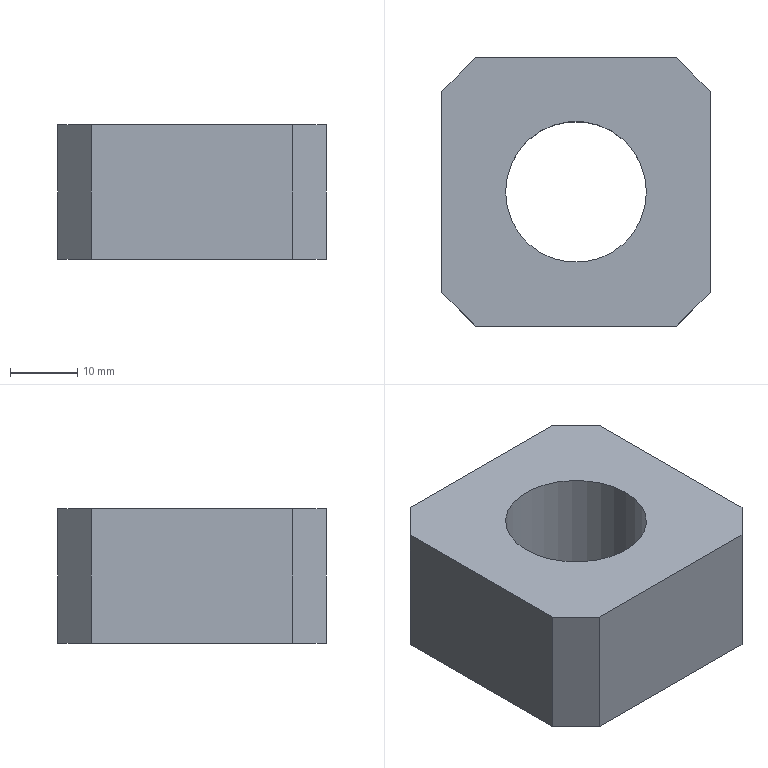NC program | NX | posted with a generic post | part box 40 x 40 x 20 mm
Whole program:
N10 G17 G21 G94 G90
(PLANAR_MILL , TOOL : D50面刀)
N12 T01 M6
N14 G54
N16 G17 G0 G90 X55. Y0. S2000 M3
N18 G43 Z30. H1
N20 Z2.1
N22 G94 G1 Z0.1 F800.
N24 X15.
N26 X-15.
N28 X-55.
N30 Z2.1
N32 G0 Z30.
(PLANAR_MILL_COPY_1 , TOOL : D50面刀)
N34 X55.
N36 Z2.
N38 G1 Z0.
N40 X15.
N42 X-15.
N44 X-55.
N46 Z2.
N48 G0 Z30.
N50 M5
(DRILLING , TOOL : D8倒角刀)
N52 T02 M6
N54 G54
N56 G17 G0 G90 X0. Y0. S2000 M3
N58 G43 Z30. H2
N60 G94 G81 G99 Z-1.5 F150. R3.
N62 G80
N64 G0 X0. Y0. Z30.
N66 M5
(DRILLING_COPY , TOOL : D15钻头)
N68 T08 M6
N70 G54
N72 G17 G0 G90 X0. Y0. S800 M3
N74 G43 Z30. H8
N76 G94 G83 G99 Z-28. F40. Q1.5 R3.
N78 G80
N80 G0 X0. Y0. Z30.
N82 M5
(ADAPTIVE_MILLING , TOOL : D10开粗)
N84 T05 M6
N86 G54
N88 G17 G0 G90 X-4.103 Y-1.849 S3500 M3
N90 G43 Z30. H5
N92 Z5.
N94 G94 G3 X-4.103 Y-1.849 Z4.506 I4.102 J1.849 F1500.
N96 X-4.103 Y-1.849 Z4.013 I4.102 J1.849
N98 X-4.103 Y-1.849 Z3.519 I4.102 J1.849
N100 X-4.103 Y-1.849 Z3.026 I4.102 J1.849
N102 X-4.103 Y-1.849 Z2.532 I4.102 J1.849
N104 X-4.103 Y-1.849 Z2.039 I4.102 J1.849
N106 X-4.103 Y-1.849 Z1.545 I4.102 J1.849
N108 X-4.103 Y-1.849 Z1.052 I4.102 J1.849
N110 X-4.103 Y-1.849 Z0.558 I4.102 J1.849
N112 X-4.103 Y-1.849 Z0.065 I4.102 J1.849
N114 X-4.103 Y-1.849 Z-0.429 I4.102 J1.849
N116 X-4.103 Y-1.849 Z-0.922 I4.102 J1.849
N118 X-4.103 Y-1.849 Z-1.416 I4.102 J1.849
N120 X-4.103 Y-1.849 Z-1.909 I4.102 J1.849
N122 X-4.103 Y-1.849 Z-2.403 I4.102 J1.849
N124 X-4.103 Y-1.849 Z-2.896 I4.102 J1.849
N126 X-4.103 Y-1.849 Z-3.39 I4.102 J1.849
N128 X-4.103 Y-1.849 Z-3.884 I4.102 J1.849
N130 X-4.103 Y-1.849 Z-4.377 I4.102 J1.849
N132 X-4.103 Y-1.849 Z-4.871 I4.102 J1.849
N134 X-4.103 Y-1.849 Z-5.364 I4.102 J1.849
N136 X-4.103 Y-1.849 Z-5.858 I4.102 J1.849
N138 X-4.103 Y-1.849 Z-6.351 I4.102 J1.849
N140 X-4.103 Y-1.849 Z-6.845 I4.102 J1.849
N142 X-4.103 Y-1.849 Z-7.338 I4.102 J1.849
N144 X-4.103 Y-1.849 Z-7.832 I4.102 J1.849
N146 X-4.103 Y-1.849 Z-8.325 I4.102 J1.849
N148 X-4.103 Y-1.849 Z-8.819 I4.102 J1.849
N150 X-4.103 Y-1.849 Z-9.312 I4.102 J1.849
N152 X-4.103 Y-1.849 Z-9.806 I4.102 J1.849
N154 X-4.103 Y-1.849 Z-10.299 I4.102 J1.849
N156 X-4.103 Y-1.849 Z-10.793 I4.102 J1.849
N158 X-4.103 Y-1.849 Z-11.287 I4.102 J1.849
N160 X4.5 Y0. Z-11.5 R4.5
N162 X-1.93 Y-4.122 R-4.525
N164 X-2.463 Y3.945 R-4.601
N166 X4.556 Y-1.177 R-4.676
N168 X-3.713 Y3.018 R4.738
N170 X4.715 Y-1.086 R-4.81
N172 X-4.329 Y2.337 R4.876
N174 X4.889 Y-0.92 R-4.945
N176 X-4.752 Y1.716 R5.012
N178 X5.026 Y-0.918 R-5.08
N180 X-4.979 Y1.453 R5.147
N182 X5.215 Y-0.596 R-5.217
N184 X-5.315 Y0.355 R-5.288
N186 X5.395 Y0.067 R-5.36
N188 X-5.354 Y-1.115 R-5.433
N190 G1 X-5.147 Y-1.855
N192 G3 X5.238 Y-1.634 R5.48
N194 X3.996 Y3.765 R5.545
N196 X-0.478 Y5.47 R5.602
N198 X-4.148 Y3.597 R5.635
N200 X-5.196 Y-1.775 R5.556
N202 X-2.419 Y-4.93 R5.621
N204 X4.314 Y-3.398 R5.531
N206 X5.266 Y-1.559 R6.154
N208 X4.289 Y-0.225 R1.01
N210 G1 X2.974 Y-0.252
N212 X2.824 Y-0.255 Z-11.496
N214 X2.674 Y-0.258 Z-11.485
N216 X2.524 Y-0.261 Z-11.466
N218 X2.374 Y-0.264 Z-11.439
N220 X2.224 Y-0.267 Z-11.405
N222 X2.074 Y-0.27 Z-11.362
N224 X1.924 Y-0.273 Z-11.31
N226 X1.774 Y-0.276 Z-11.25
N228 X1.624 Y-0.279 Z-11.179
N230 X1.474 Y-0.282 Z-11.098
N232 X1.324 Y-0.285 Z-11.005
N234 X1.174 Y-0.288 Z-10.9
N236 X1.024 Y-0.291 Z-10.78
N238 X0.875 Y-0.294 Z-10.642
N240 X0.725 Y-0.297 Z-10.484
N242 X0.575 Y-0.3 Z-10.3
N244 X0.425 Y-0.303 Z-10.08
N246 X0.275 Y-0.306 Z-9.808
N248 X0.125 Y-0.309 Z-9.437
N250 X-0.025 Y-0.312 Z-8.5
N252 G0 Z30.
N254 X-4.102 Y-1.849
N256 Z-8.5
N258 G3 X-4.102 Y-1.849 Z-8.994 I4.102 J1.849
N260 X-4.102 Y-1.849 Z-9.487 I4.102 J1.849
N262 X-4.102 Y-1.849 Z-9.981 I4.102 J1.849
N264 X-4.102 Y-1.849 Z-10.474 I4.102 J1.849
N266 X-4.102 Y-1.849 Z-10.968 I4.102 J1.849
N268 X-4.102 Y-1.849 Z-11.461 I4.102 J1.849
N270 X-4.102 Y-1.849 Z-11.955 I4.102 J1.849
N272 X-4.102 Y-1.849 Z-12.448 I4.102 J1.849
N274 X-4.102 Y-1.849 Z-12.942 I4.102 J1.849
N276 X-4.102 Y-1.849 Z-13.435 I4.102 J1.849
N278 X-4.102 Y-1.849 Z-13.929 I4.102 J1.849
N280 X-4.102 Y-1.849 Z-14.422 I4.102 J1.849
N282 X-4.102 Y-1.849 Z-14.916 I4.102 J1.849
N284 X-4.102 Y-1.849 Z-15.409 I4.102 J1.849
N286 X-4.102 Y-1.849 Z-15.903 I4.102 J1.849
N288 X-4.102 Y-1.849 Z-16.396 I4.102 J1.849
N290 X-4.102 Y-1.849 Z-16.89 I4.102 J1.849
N292 X-4.102 Y-1.849 Z-17.384 I4.102 J1.849
N294 X-4.102 Y-1.849 Z-17.877 I4.102 J1.849
N296 X-4.102 Y-1.849 Z-18.371 I4.102 J1.849
N298 X-4.102 Y-1.849 Z-18.864 I4.102 J1.849
N300 X-4.102 Y-1.849 Z-19.358 I4.102 J1.849
N302 X-4.102 Y-1.849 Z-19.851 I4.102 J1.849
N304 X-4.102 Y-1.849 Z-20.345 I4.102 J1.849
N306 X-4.102 Y-1.849 Z-20.838 I4.102 J1.849
N308 X-4.102 Y-1.849 Z-21.332 I4.102 J1.849
N310 X-4.102 Y-1.849 Z-21.825 I4.102 J1.849
N312 X-4.102 Y-1.849 Z-22.319 I4.102 J1.849
N314 X-4.102 Y-1.849 Z-22.812 I4.102 J1.849
N316 X-4.102 Y-1.849 Z-23.306 I4.102 J1.849
N318 X-4.102 Y-1.849 Z-23.799 I4.102 J1.849
N320 X-4.102 Y-1.849 Z-24.293 I4.102 J1.849
N322 X-4.102 Y-1.849 Z-24.787 I4.102 J1.849
N324 X4.501 Y0.001 Z-25. R4.5
N326 X-1.929 Y-4.121 R-4.525
N328 X-2.463 Y3.946 R-4.601
N330 X4.557 Y-1.176 R-4.677
N332 X-3.859 Y2.83 R4.74
N334 X4.716 Y-1.086 R-4.811
N336 X-4.327 Y2.337 R4.876
N338 X4.89 Y-0.919 R-4.945
N340 X-4.751 Y1.717 R5.012
N342 X5.027 Y-0.918 R-5.08
N344 X-5.042 Y1.213 R5.148
N346 X5.216 Y-0.596 R-5.217
N348 X-5.313 Y0.357 R-5.288
N350 X5.39 Y-0.188 R-5.359
N352 X-5.455 Y-0.352 R-5.43
N354 X-5.227 Y-1.61 R6.565
N356 X5.463 Y-0.563 R5.482
N358 X-0.478 Y5.47 R5.504
N360 X-4.148 Y3.597 R5.635
N362 X-5.196 Y-1.775 R5.556
N364 X-2.419 Y-4.93 R5.621
N366 X4.328 Y-3.381 R5.531
N368 G1 X4.825 Y-2.621
N370 G3 X4.153 Y-1.155 R1.01
N372 G1 X2.863 Y-0.872
N374 X2.716 Y-0.84 Z-24.996
N376 X2.57 Y-0.808 Z-24.985
N378 X2.423 Y-0.776 Z-24.966
N380 X2.277 Y-0.744 Z-24.939
N382 X2.13 Y-0.711 Z-24.905
N384 X1.983 Y-0.679 Z-24.862
N386 X1.837 Y-0.647 Z-24.81
N388 X1.69 Y-0.615 Z-24.75
N390 X1.544 Y-0.583 Z-24.679
N392 X1.397 Y-0.55 Z-24.598
N394 X1.251 Y-0.518 Z-24.505
N396 X1.104 Y-0.486 Z-24.4
N398 X0.958 Y-0.454 Z-24.28
N400 X0.811 Y-0.422 Z-24.142
N402 X0.665 Y-0.39 Z-23.984
N404 X0.518 Y-0.357 Z-23.8
N406 X0.372 Y-0.325 Z-23.58
N408 X0.225 Y-0.293 Z-23.308
N410 X0.079 Y-0.261 Z-22.937
N412 X-0.068 Y-0.229 Z-22.
N414 G0 Z30.
(ADAPTIVE_MILLING_COPY , TOOL : D10开粗)
N416 X0.006 Y-29.505
N418 Z-18.
N420 G1 Z-21.
N422 G3 X0.006 Y-27.505 R1.046
N424 X-3.063 Y-27.242 R16.364
N426 X-10.78 Y-27.2 R616.908
N428 G1 X-21.13 Y-27.189
N430 G2 X-25.367 Y-24.645 R5.736
N432 X-26.921 Y-20.308 R9.763
N434 X-27.19 Y-14.469 R47.531
N436 G1 X-27.199 Y-8.956
N438 X-27.197 Y20.955
N440 G2 X-24.769 Y25.282 R5.653
N442 X-20.42 Y26.906 R9.551
N444 X-14.881 Y27.188 R43.135
N446 G1 X-8.956 Y27.2
N448 X20.958 Y27.198
N450 G2 X25.262 Y24.798 R5.647
N452 X26.889 Y20.531 R9.44
N454 X27.187 Y14.919 R41.497
N456 G1 X27.2 Y8.919
N458 Y-20.904
N460 G2 X24.806 Y-25.25 R5.644
N462 X20.534 Y-26.886 R9.415
N464 X14.922 Y-27.186 R41.396
N466 G1 X1.483 Y-27.185
N468 G3 X-8.801 Y-26.903 R141.138
N470 G2 X-19.668 Y-26.88 R700.527
N472 X-25.157 Y-23.343 R6.987
N474 X-26.615 Y-18.684 R11.927
N476 X-26.886 Y-12.694 R53.51
N478 G1 X-26.899 Y-6.619
N480 X-26.897 Y19.268
N482 G2 X-23.398 Y25.126 R6.947
N484 X-18.639 Y26.622 R11.91
N486 X-12.798 Y26.886 R53.435
N488 G1 X-6.948 Y26.9
N490 X19.267 Y26.898
N492 G2 X25.127 Y23.397 R6.945
N494 X26.627 Y18.602 R11.944
N496 X26.885 Y12.836 R53.695
N498 G1 X26.899 Y7.061
N500 Y-19.254
N502 G2 X23.426 Y-25.106 R6.946
N504 X18.746 Y-26.606 R11.775
N506 X12.568 Y-26.886 R53.616
N508 G1 X6.193 Y-26.899
N510 X-12.029 Y-26.897
N512 G3 X-15.809 Y-26.628 R22.26
N514 G2 X-18.944 Y-26.534 R33.644
N516 X-24.922 Y-22.293 R7.837
N518 X-26.328 Y-17.302 R13.761
N520 X-26.586 Y-10.898 R64.094
N522 G1 X-26.599 Y-4.373
N524 X-26.597 Y17.802
N526 G2 X-22.255 Y24.943 R7.848
N528 X-17.226 Y26.337 R13.883
N530 X-10.896 Y26.587 R65.463
N532 G1 X-4.371 Y26.6
N534 X17.842 Y26.598
N536 G2 X24.949 Y22.245 R7.847
N538 X26.326 Y17.326 R13.779
N540 X26.589 Y10.547 R66.976
N542 G1 X26.599 Y4.322
N544 X26.598 Y-17.829
N546 G2 X22.183 Y-24.978 R7.864
N548 X17.105 Y-26.348 R14.148
N550 X10.512 Y-26.588 R70.967
N552 G1 X3.912 Y-26.598
N554 X-12.051 Y-26.597
N556 G3 X-17.189 Y-26.312 R60.447
N558 G2 X-24.731 Y-21.258 R8.562
N560 X-26.045 Y-16.049 R15.639
N562 X-26.29 Y-8.705 R82.022
N564 G1 X-26.298 Y-3.38
N566 X-26.297 Y16.529
N568 G2 X-25.012 Y21.468 R9.037
N570 X-20.079 Y25.215 R9.315
N572 X-14.627 Y26.158 R20.171
N574 X-6.004 Y26.298 R170.126
N576 G1 X16.267 Y26.299
N578 G2 X20.613 Y25.48 R9.785
N580 X24.989 Y20.674 R8.889
N582 X26.112 Y15.3 R17.702
N584 X26.297 Y6.604 R130.191
N586 G1 X26.299 Y2.779
N588 X26.298 Y-16.554
N590 G2 X24.916 Y-21.615 R8.967
N592 X20.075 Y-25.213 R9.361
N594 X14.81 Y-26.145 R19.841
N596 X7.013 Y-26.295 R142.478
N598 G1 X2.588 Y-26.298
N600 X-12.025
N602 G3 X-16.748 Y-26.003 R283.987
N604 G2 X-24.364 Y-20.653 R9.084
N606 X-25.713 Y-15.372 R16.269
N608 X-25.988 Y-7.805 R79.761
N610 G1 X-25.998 Y-1.355
N612 X-25.996 Y15.329
N614 G2 X-25.22 Y19.766 R10.975
N616 X-20.274 Y24.532 R9.224
N618 X-14.885 Y25.762 R17.475
N620 X-7.241 Y25.991 R95.528
N622 G1 X-1.391 Y25.999
N624 X15.292 Y25.998
N626 G2 X19.697 Y25.251 R11.093
N628 X24.521 Y20.3 R9.207
N630 X25.756 Y14.951 R17.346
N632 X25.991 Y7.307 R93.356
N634 G1 X25.999 Y1.382
N636 X25.997 Y-15.317
N638 G2 X25.254 Y-19.685 R11.055
N640 X20.355 Y-24.494 R9.19
N642 X14.972 Y-25.752 R17.227
N644 X7.778 Y-25.987 R87.466
N646 G1 X1.253 Y-25.998
N648 X-12.029 Y-25.996
N650 G2 X-16.206 Y-25.704 R147.203
N652 X-24.091 Y-19.91 R9.578
N654 X-25.426 Y-14.356 R17.648
N656 X-25.684 Y-7.126 R83.895
N658 G1 X-25.698 Y-0.151
N660 X-25.696 Y14.242
N662 G2 X-25.094 Y18.603 R13.05
N664 X-19.914 Y24.08 R9.477
N666 X-14.363 Y25.426 R17.51
N668 X-6.983 Y25.686 R84.677
N670 G1 X-0.158 Y25.699
N672 X14.241 Y25.697
N674 G2 X18.603 Y25.095 R13.048
N676 X24.071 Y19.935 R9.472
N678 X25.412 Y14.498 R17.283
N680 X25.688 Y6.668 R85.392
N682 G1 X25.699 Y0.143
N684 X25.697 Y-14.191
N686 G2 X25.134 Y-18.485 R13.32
N688 X19.965 Y-24.054 R9.454
N690 X14.379 Y-25.422 R17.412
N692 X6.361 Y-25.688 R90.585
N694 G1 X1.036 Y-25.697
N696 X-12.039 Y-25.696
N698 G2 X-16.229 Y-25.319 R39.844
N700 X-23.718 Y-19.426 R9.943
N702 X-24.382 Y-17.674 R24.511
N704 G1 X-24.758 Y-16.969
N706 G2 X-25.152 Y-14.963 R6.081
N708 X-25.396 Y-1.539 R247.799
N710 G1 X-25.397 Y12.699
N712 G2 X-25.073 Y16.915 R19.108
N714 X-19.631 Y23.607 R9.704
N716 X-17.713 Y24.361 R18.68
N718 G1 X-16.969 Y24.758
N720 G2 X-14.962 Y25.152 R6.082
N722 X-1.54 Y25.397 R246.646
N724 G1 X12.648 Y25.398
N726 G2 X16.755 Y25.109 R20.046
N728 X23.635 Y19.574 R9.715
N730 X24.359 Y17.716 R19.282
N732 G1 X24.758 Y16.969
N734 G2 X25.152 Y14.962 R6.082
N736 X25.397 Y1.552 R246.781
N738 G1 X25.398 Y-12.648
N740 G2 X25.084 Y-16.865 R19.507
N742 X19.573 Y-23.632 R9.717
N744 X17.724 Y-24.356 R19.997
N746 G1 X16.969 Y-24.758
N748 G2 X14.962 Y-25.152 R6.082
N750 X1.25 Y-25.396 R254.829
N752 G1 X-12.012 Y-25.397
N754 G2 X-16.117 Y-25.03 R87.651
N756 X-23.285 Y-19.148 R10.674
N758 G3 X-23.642 Y-18.641 R1.667
N760 G2 X-24.758 Y-16.969 R6.011
N762 X-25.15 Y-15. R5.999
N764 G1 Y15.001
N766 G2 X-24.757 Y16.972 R5.996
N768 X-19.261 Y23.213 R10.678
N770 G3 X-18.641 Y23.642 R1.867
N772 G2 X-17.694 Y24.371 R5.875
N774 G3 X-17.657 Y26.114 R1.
N776 X-18.4 Y26.23 Z-20.961 R1.061
N778 G1 X-19.608 Y26.057 Z-20.9
N780 X-21.474 Y25.791 F15000.
N782 G3 X-22.018 Y25.53 R1.009
N784 G1 X-26.995 Y20.849
N786 G3 X-27.28 Y19.877 R1.001
N788 G1 X-26.883 Y18.294
N790 X-26.587 Y17.132 Z-20.96 F1500.
N792 G3 X-26.086 Y16.549 Z-21. R1.
N794 X-24.757 Y16.972 R1.
N796 G2 X-20.031 Y22.255 R13.615
N798 G1 X-18.783 Y23.5
N800 G3 X-18.774 Y24.905 R1.
N802 X-19.664 Y25.196 Z-20.951 R1.041
N804 G1 X-20.678 Y25.114 Z-20.9
N806 X-22.461 Y24.969 F15000.
N808 G3 X-23.107 Y24.658 R1.005
N810 G1 X-25.44 Y22.186
N812 G3 X-25.706 Y21.613 R1.008
N814 G1 X-25.911 Y19.808
N816 X-26.051 Y18.545 Z-20.964 F1500.
N818 G3 X-25.838 Y17.875 Z-21. R1.001
N820 X-24.281 Y17.862 R1.
N822 G1 X-23.641 Y18.642
N824 X-18.641 Y23.642
N826 G2 X-16.969 Y24.758 R5.996
N828 X-14.999 Y25.15 R5.998
N830 G1 X15.001
N832 G2 X16.972 Y24.757 R5.996
N834 X21.083 Y22.247 R10.697
N836 X22.188 Y21.11 R16.296
N838 X23.493 Y18.812 R20.49
N840 G1 X24.283 Y17.86
N842 X24.371 Y17.694
N844 G3 X26.114 Y17.657 R1.
N846 X26.23 Y18.4 Z-20.961 R1.061
N848 G1 X26.057 Y19.608 Z-20.9
N850 X25.791 Y21.474 F15000.
N852 G3 X25.53 Y22.018 R1.009
N854 G1 X20.849 Y26.995
N856 G3 X19.877 Y27.28 R1.001
N858 G1 X18.294 Y26.883
N860 X17.132 Y26.587 Z-20.96 F1500.
N862 G3 X16.549 Y26.086 Z-21. R1.
N864 X16.972 Y24.757 R1.
N866 G2 X22.404 Y19.879 R14.044
N868 G1 X23.597 Y18.686
N870 G3 X25.002 Y18.677 R1.
N872 X25.293 Y19.567 Z-20.951 R1.041
N874 G1 X25.211 Y20.581 Z-20.9
N876 X25.065 Y22.364 F15000.
N878 G3 X24.756 Y23.01 R1.005
N880 G1 X22.186 Y25.44
N882 G3 X21.612 Y25.707 R1.008
N884 G1 X19.807 Y25.912
N886 X18.544 Y26.051 Z-20.964 F1500.
N888 G3 X17.875 Y25.837 Z-21. R1.001
N890 X17.862 Y24.281 R1.
N892 G1 X18.642 Y23.641
N894 X23.642 Y18.641
N896 G2 X24.758 Y16.969 R5.996
N898 X25.15 Y14.999 R5.998
N900 G1 Y-15.001
N902 G2 X24.757 Y-16.972 R5.996
N904 X19.259 Y-23.211 R10.684
N906 G3 X18.641 Y-23.642 R1.859
N908 G2 X17.694 Y-24.371 R5.875
N910 G3 X17.657 Y-26.114 R1.
N912 X18.4 Y-26.23 Z-20.961 R1.061
N914 G1 X19.608 Y-26.057 Z-20.9
N916 X21.474 Y-25.791 F15000.
N918 G3 X22.018 Y-25.53 R1.009
N920 G1 X26.995 Y-20.849
N922 G3 X27.28 Y-19.877 R1.001
N924 G1 X26.883 Y-18.294
N926 X26.587 Y-17.132 Z-20.96 F1500.
N928 G3 X26.086 Y-16.549 Z-21. R1.
N930 X24.757 Y-16.972 R1.
N932 G2 X20.045 Y-22.242 R13.595
N934 G1 X18.771 Y-23.512
N936 G3 X18.761 Y-24.917 R1.
N938 X19.651 Y-25.209 Z-20.951 R1.041
N940 G1 X20.665 Y-25.126 Z-20.9
N942 X22.448 Y-24.981 F15000.
N944 G3 X23.094 Y-24.671 R1.005
N946 G1 X25.44 Y-22.186
N948 G3 X25.706 Y-21.613 R1.008
N950 G1 X25.911 Y-19.808
N952 X26.051 Y-18.545 Z-20.964 F1500.
N954 G3 X25.838 Y-17.875 Z-21. R1.001
N956 X24.281 Y-17.862 R1.
N958 G1 X23.641 Y-18.642
N960 X18.641 Y-23.642
N962 G2 X16.969 Y-24.758 R5.996
N964 X14.999 Y-25.15 R5.998
N966 G1 X-15.001
N968 G2 X-16.972 Y-24.757 R5.996
N970 X-22.334 Y-19.949 R13.908
N972 G1 X-23.528 Y-18.755
N974 G3 X-24.933 Y-18.746 R1.
N976 X-25.224 Y-19.636 Z-20.951 R1.041
N978 G1 X-25.141 Y-20.65 Z-20.9
N980 X-24.996 Y-22.433 F15000.
N982 G3 X-24.686 Y-23.079 R1.005
N984 G1 X-22.186 Y-25.44
N986 G3 X-21.612 Y-25.706 R1.008
N988 G1 X-19.808 Y-25.911
N990 X-18.545 Y-26.051 Z-20.964 F1500.
N992 G3 X-17.875 Y-25.838 Z-21. R1.001
N994 X-17.862 Y-24.281 R1.
N996 G1 X-18.642 Y-23.641
N998 X-22.354 Y-19.929
N1000 G3 X-23.733 Y-19.882 R1.01
N1002 G1 X-24.899 Y-20.901
N1004 X-25.012 Y-20.999 Z-20.996
N1006 X-25.125 Y-21.098 Z-20.985
N1008 X-25.238 Y-21.197 Z-20.966
N1010 X-25.351 Y-21.295 Z-20.939
N1012 X-25.464 Y-21.394 Z-20.905
N1014 X-25.577 Y-21.493 Z-20.862
N1016 X-25.69 Y-21.591 Z-20.81
N1018 X-25.803 Y-21.69 Z-20.75
N1020 X-25.916 Y-21.789 Z-20.679
N1022 X-26.029 Y-21.887 Z-20.598
N1024 X-26.142 Y-21.986 Z-20.505
N1026 X-26.255 Y-22.085 Z-20.4
N1028 X-26.368 Y-22.183 Z-20.28
N1030 X-26.481 Y-22.282 Z-20.142
N1032 X-26.594 Y-22.381 Z-19.984
N1034 X-26.707 Y-22.479 Z-19.8
N1036 X-26.82 Y-22.578 Z-19.58
N1038 X-26.933 Y-22.677 Z-19.308
N1040 X-27.046 Y-22.775 Z-18.937
N1042 X-27.159 Y-22.874 Z-18.
N1044 G0 Z30.
N1046 M5
(PLANAR_MILL_1_COPY_1 , TOOL : D10精光)
N1048 T07 M6
N1050 G54
N1052 G17 G0 G90 X2.872 Y-2. S2500 M3
N1054 G43 Z30. H7
N1056 Z-19.
N1058 G94 G1 Z-21. F400.
N1060 X3.5
N1062 G3 X5.5 Y0. R2.
N1064 X0. Y5.5 R5.5
N1066 X5.5 Y0. R-5.5
N1068 X3.5 Y2. R2.
N1070 G1 X2.872
N1072 Z-19.
N1074 G0 Z30.
(PLANAR_MILL_1 , TOOL : D10精光)
N1076 X-15.071 Y-27.
N1078 Z-19.
N1080 G1 Z-21. F600.
N1082 X-18.536 Y-23.535
N1084 X-23.536 Y-18.536
N1086 G2 X-25. Y-15. R5.
N1088 G1 Y15.
N1090 G2 X-23.536 Y18.536 R5.
N1092 G1 X-18.536 Y23.536
N1094 G2 X-15. Y25. R5.
N1096 G1 X15.
N1098 G2 X18.536 Y23.536 R5.
N1100 G1 X23.536 Y18.536
N1102 G2 X25. Y15. R5.
N1104 G1 Y-15.
N1106 G2 X23.536 Y-18.536 R5.
N1108 G1 X18.536 Y-23.536
N1110 G2 X15. Y-25. R5.
N1112 G1 X-14.999
N1114 X-19.899
N1116 Z-19.
N1118 G0 Z30.
N1120 X-15.071 Y-27.
N1122 Z-19.
N1124 G1 Z-21.
N1126 X-18.536 Y-23.535
N1128 X-23.536 Y-18.536
N1130 G2 X-25. Y-15. R5.
N1132 G1 Y15.
N1134 G2 X-23.536 Y18.536 R5.
N1136 G1 X-18.536 Y23.536
N1138 G2 X-15. Y25. R5.
N1140 G1 X15.
N1142 G2 X18.536 Y23.536 R5.
N1144 G1 X23.536 Y18.536
N1146 G2 X25. Y15. R5.
N1148 G1 Y-15.
N1150 G2 X23.536 Y-18.536 R5.
N1152 G1 X18.536 Y-23.536
N1154 G2 X15. Y-25. R5.
N1156 G1 X-14.999
N1158 X-19.899
N1160 Z-19.
N1162 G0 Z30.
N1164 M5
(PLANAR_MILL_1_COPY , TOOL : D8倒角刀)
N1166 T02 M6
N1168 G54
N1170 G17 G0 G90 X-14.036 Y-24.5 S2500 M3
N1172 G43 Z30. H2
N1174 Z-0.5
N1176 G94 G1 Z-2.5 F600.
N1178 X-16.768 Y-21.767
N1180 X-21.768 Y-16.768
N1182 G2 X-22.5 Y-15. R2.5
N1184 G1 Y15.
N1186 G2 X-21.768 Y16.768 R2.5
N1188 G1 X-16.768 Y21.768
N1190 G2 X-15. Y22.5 R2.5
N1192 G1 X15.
N1194 G2 X16.768 Y21.768 R2.5
N1196 G1 X21.768 Y16.768
N1198 G2 X22.5 Y15. R2.5
N1200 G1 Y-15.
N1202 G2 X21.768 Y-16.768 R2.5
N1204 G1 X16.768 Y-21.768
N1206 G2 X15. Y-22.5 R2.5
N1208 G1 X-14.999
N1210 X-18.864
N1212 Z-0.5
N1214 G0 Z30.
(PLANAR_MILL_1_COPY_COPY , TOOL : D8倒角刀)
N1216 X6.29 Y-2. S3000
N1218 Z-0.5
N1220 G1 Z-2.5
N1222 X6.6
N1224 G3 X8.6 Y0. R2.
N1226 X0. Y8.6 R8.6
N1228 X8.6 Y0. R-8.6
N1230 X6.6 Y2. R2.
N1232 G1 X7.1 Y-2.
N1234 G3 X9.1 Y0. R2.
N1236 X0. Y9.1 R9.1
N1238 X9.1 Y0. R-9.1
N1240 X7.1 Y2. R2.
N1242 G1 X7.6 Y-2.
N1244 G3 X9.6 Y0. R2.
N1246 X0. Y9.6 R9.6
N1248 X9.6 Y0. R-9.6
N1250 X7.6 Y2. R2.
N1252 G1 X7.332
N1254 Z-0.5
N1256 G0 Z30.
N1258 M5
(THREAD_MILLING , TOOL : THREAD_MILL)
N1260 T09 M6
N1262 G54
N1264 G17 G0 G90 X0. Y0. S2500 M3
N1266 G43 Z30. H9
N1268 Z-24.75
N1270 G41 G94 G3 X0.3 Y0. Z-24. I0.15 J0. F200. D9
N1272 X0.3 Y0. Z-21. I-0.3 J0.
N1274 X0.3 Y0. Z-18. I-0.3 J0.
N1276 X0.3 Y0. Z-15. I-0.3 J0.
N1278 X0.3 Y0. Z-12. I-0.3 J0.
N1280 X0.3 Y0. Z-9. I-0.3 J0.
N1282 X0.3 Y0. Z-6. I-0.3 J0.
N1284 X0.3 Y0. Z-3. I-0.3 J0.
N1286 X0.3 Y0. Z0. I-0.3 J0.
N1288 X-0.15 Y0.26 Z1. R0.3
N1290 X0. Y0. Z1.75 I0.075 J-0.13
N1292 G40
N1294 G0 Z-24.75
N1296 G41 G3 X0.4 Y0. Z-24. I0.2 J0.
N1298 X0.4 Y0. Z-21. I-0.4 J0.
N1300 X0.4 Y0. Z-18. I-0.4 J0.
N1302 X0.4 Y0. Z-15. I-0.4 J0.
N1304 X0.4 Y0. Z-12. I-0.4 J0.
N1306 X0.4 Y0. Z-9. I-0.4 J0.
N1308 X0.4 Y0. Z-6. I-0.4 J0.
N1310 X0.4 Y0. Z-3. I-0.4 J0.
N1312 X0.4 Y0. Z0. I-0.4 J0.
N1314 X-0.2 Y0.346 Z1. R0.4
N1316 X0. Y0. Z1.75 I0.1 J-0.173
N1318 G40
N1320 G0 Z-24.75
N1322 G41 G3 X0.5 Y0. Z-24. I0.25 J0.
N1324 X0.5 Y0. Z-21. I-0.5 J0.
N1326 X0.5 Y0. Z-18. I-0.5 J0.
N1328 X0.5 Y0. Z-15. I-0.5 J0.
N1330 X0.5 Y0. Z-12. I-0.5 J0.
N1332 X0.5 Y0. Z-9. I-0.5 J0.
N1334 X0.5 Y0. Z-6. I-0.5 J0.
N1336 X0.5 Y0. Z-3. I-0.5 J0.
N1338 X0.5 Y0. Z0. I-0.5 J0.
N1340 X-0.25 Y0.433 Z1. R0.5
N1342 X0. Y0. Z1.75 I0.125 J-0.217
N1344 G40
N1346 G0 Z-24.137
N1348 G41 G1 X0.488 Y-0.107
N1350 X0.545 Y-0.097 Z-24.092
N1352 X0.587 Y-0.056 Z-24.046
N1354 X0.6 Y0. Z-24.
N1356 G3 X0.6 Y0. Z-21. I-0.6 J0.
N1358 X0.6 Y0. Z-18. I-0.6 J0.
N1360 X0.6 Y0. Z-15. I-0.6 J0.
N1362 X0.6 Y0. Z-12. I-0.6 J0.
N1364 X0.6 Y0. Z-9. I-0.6 J0.
N1366 X0.6 Y0. Z-6. I-0.6 J0.
N1368 X0.6 Y0. Z-3. I-0.6 J0.
N1370 X0.6 Y0. Z0. I-0.6 J0.
N1372 X-0.3 Y0.52 Z1. R0.6
N1374 G1 X-0.343 Y0.481 Z1.046
N1376 X-0.357 Y0.424 Z1.092
N1378 X-0.337 Y0.369 Z1.137
N1380 G40
N1382 X0. Y0.
N1384 G0 Z-24.239
N1386 G41 G1 X0.462 Y-0.191
N1388 G3 X0.7 Y0. Z-24. R0.196
N1390 X0.7 Y0. Z-21. I-0.7 J0.
N1392 X0.7 Y0. Z-18. I-0.7 J0.
N1394 X0.7 Y0. Z-15. I-0.7 J0.
N1396 X0.7 Y0. Z-12. I-0.7 J0.
N1398 X0.7 Y0. Z-9. I-0.7 J0.
N1400 X0.7 Y0. Z-6. I-0.7 J0.
N1402 X0.7 Y0. Z-3. I-0.7 J0.
N1404 X0.7 Y0. Z0. I-0.7 J0.
N1406 X-0.35 Y0.606 Z1. R0.7
N1408 X-0.397 Y0.305 Z1.239 R0.196
N1410 G40
N1412 G1 X0. Y0.
N1414 G0 Z-24.315
N1416 G41 G1 X0.43 Y-0.256
N1418 G3 X0.8 Y0. Z-24. R0.273
N1420 X0.8 Y0. Z-21. I-0.8 J0.
N1422 X0.8 Y0. Z-18. I-0.8 J0.
N1424 X0.8 Y0. Z-15. I-0.8 J0.
N1426 X0.8 Y0. Z-12. I-0.8 J0.
N1428 X0.8 Y0. Z-9. I-0.8 J0.
N1430 X0.8 Y0. Z-6. I-0.8 J0.
N1432 X0.8 Y0. Z-3. I-0.8 J0.
N1434 X0.8 Y0. Z0. I-0.8 J0.
N1436 X-0.4 Y0.693 Z1. R0.8
N1438 X-0.436 Y0.244 Z1.315 R0.273
N1440 G40
N1442 G1 X0. Y0.
N1444 G0 Z-24.375
N1446 G41 G1 X0.396 Y-0.305
N1448 G3 X0.9 Y0. Z-24. R0.344
N1450 X0.9 Y0. Z-21. I-0.9 J0.
N1452 X0.9 Y0. Z-18. I-0.9 J0.
N1454 X0.9 Y0. Z-15. I-0.9 J0.
N1456 X0.9 Y0. Z-12. I-0.9 J0.
N1458 X0.9 Y0. Z-9. I-0.9 J0.
N1460 X0.9 Y0. Z-6. I-0.9 J0.
N1462 X0.9 Y0. Z-3. I-0.9 J0.
N1464 X0.9 Y0. Z0. I-0.9 J0.
N1466 X-0.45 Y0.779 Z1. R0.9
N1468 X-0.462 Y0.19 Z1.375 R0.344
N1470 G40
N1472 G1 X0. Y0.
N1474 G0 Z-24.422
N1476 G41 G1 X0.364 Y-0.343
N1478 G3 X1. Y0. Z-24. R0.411
N1480 X1. Y0. Z-21. I-1. J0.
N1482 X1. Y0. Z-18. I-1. J0.
N1484 X1. Y0. Z-15. I-1. J0.
N1486 X1. Y0. Z-12. I-1. J0.
N1488 X1. Y0. Z-9. I-1. J0.
N1490 X1. Y0. Z-6. I-1. J0.
N1492 X1. Y0. Z-3. I-1. J0.
N1494 X1. Y0. Z0. I-1. J0.
N1496 X-0.5 Y0.866 Z1. R1.
N1498 X-0.479 Y0.143 Z1.422 R0.411
N1500 G40
N1502 G1 X0. Y0.
N1504 G0 Z-24.46
N1506 G41 G1 X0.334 Y-0.373
N1508 G3 X1.1 Y0. Z-24. R0.474
N1510 X1.1 Y0. Z-21. I-1.1 J0.
N1512 X1.1 Y0. Z-18. I-1.1 J0.
N1514 X1.1 Y0. Z-15. I-1.1 J0.
N1516 X1.1 Y0. Z-12. I-1.1 J0.
N1518 X1.1 Y0. Z-9. I-1.1 J0.
N1520 X1.1 Y0. Z-6. I-1.1 J0.
N1522 X1.1 Y0. Z-3. I-1.1 J0.
N1524 X1.1 Y0. Z0. I-1.1 J0.
N1526 X-0.55 Y0.953 Z1. R1.1
N1528 X-0.489 Y0.103 Z1.46 R0.474
N1530 G40
N1532 G1 X0. Y0.
N1534 G0 Z-24.491
N1536 G41 G1 X0.306 Y-0.395
N1538 G3 X1.2 Y0. Z-24. R0.535
N1540 X1.2 Y0. Z-21. I-1.2 J0.
N1542 X1.2 Y0. Z-18. I-1.2 J0.
N1544 X1.2 Y0. Z-15. I-1.2 J0.
N1546 X1.2 Y0. Z-12. I-1.2 J0.
N1548 X1.2 Y0. Z-9. I-1.2 J0.
N1550 X1.2 Y0. Z-6. I-1.2 J0.
N1552 X1.2 Y0. Z-3. I-1.2 J0.
N1554 X1.2 Y0. Z0. I-1.2 J0.
N1556 X-0.6 Y1.039 Z1. R1.2
N1558 X-0.495 Y0.067 Z1.491 R0.535
N1560 G40
N1562 G1 X0. Y0.
N1564 G0 Z-24.517
N1566 G41 G1 X0.281 Y-0.414
N1568 G3 X1.3 Y0. Z-24. R0.593
N1570 X1.3 Y0. Z-21. I-1.3 J0.
N1572 X1.3 Y0. Z-18. I-1.3 J0.
N1574 X1.3 Y0. Z-15. I-1.3 J0.
N1576 X1.3 Y0. Z-12. I-1.3 J0.
N1578 X1.3 Y0. Z-9. I-1.3 J0.
N1580 X1.3 Y0. Z-6. I-1.3 J0.
N1582 X1.3 Y0. Z-3. I-1.3 J0.
N1584 X1.3 Y0. Z0. I-1.3 J0.
N1586 X-0.65 Y1.126 Z1. R1.3
N1588 X-0.499 Y0.036 Z1.517 R0.593
N1590 G40
N1592 G1 X0. Y0.
N1594 G0 Z-24.538
N1596 G41 G1 X0.258 Y-0.428
N1598 G3 X1.4 Y0. Z-24. R0.651
N1600 X1.4 Y0. Z-21. I-1.4 J0.
N1602 X1.4 Y0. Z-18. I-1.4 J0.
N1604 X1.4 Y0. Z-15. I-1.4 J0.
N1606 X1.4 Y0. Z-12. I-1.4 J0.
N1608 X1.4 Y0. Z-9. I-1.4 J0.
N1610 X1.4 Y0. Z-6. I-1.4 J0.
N1612 X1.4 Y0. Z-3. I-1.4 J0.
N1614 X1.4 Y0. Z0. I-1.4 J0.
N1616 X-0.7 Y1.212 Z1. R1.4
N1618 X-0.5 Y0.01 Z1.538 R0.651
N1620 G40
N1622 G1 X0. Y0.
N1624 G0 Z-24.557
N1626 G41 G1 X0.238 Y-0.44
N1628 G3 X1.5 Y0. Z-24. R0.708
N1630 X1.5 Y0. Z-21. I-1.5 J0.
N1632 X1.5 Y0. Z-18. I-1.5 J0.
N1634 X1.5 Y0. Z-15. I-1.5 J0.
N1636 X1.5 Y0. Z-12. I-1.5 J0.
N1638 X1.5 Y0. Z-9. I-1.5 J0.
N1640 X1.5 Y0. Z-6. I-1.5 J0.
N1642 X1.5 Y0. Z-3. I-1.5 J0.
N1644 X1.5 Y0. Z0. I-1.5 J0.
N1646 X-0.75 Y1.299 Z1. R1.5
N1648 X-0.5 Y-0.014 Z1.557 R0.708
N1650 G40
N1652 G1 X0. Y0.
N1654 G0 Z-24.572
N1656 G41 G1 X0.22 Y-0.449
N1658 G3 X1.6 Y0. Z-24. R0.763
N1660 X1.6 Y0. Z-21. I-1.6 J0.
N1662 X1.6 Y0. Z-18. I-1.6 J0.
N1664 X1.6 Y0. Z-15. I-1.6 J0.
N1666 X1.6 Y0. Z-12. I-1.6 J0.
N1668 X1.6 Y0. Z-9. I-1.6 J0.
N1670 X1.6 Y0. Z-6. I-1.6 J0.
N1672 X1.6 Y0. Z-3. I-1.6 J0.
N1674 X1.6 Y0. Z0. I-1.6 J0.
N1676 X-0.8 Y1.386 Z1. R1.6
N1678 X-0.499 Y-0.034 Z1.572 R0.763
N1680 G40
N1682 G1 X0. Y0.
N1684 G0 Z-24.586
N1686 G41 G1 X0.203 Y-0.457
N1688 G3 X1.7 Y0. Z-24. R0.818
N1690 X1.7 Y0. Z-21. I-1.7 J0.
N1692 X1.7 Y0. Z-18. I-1.7 J0.
N1694 X1.7 Y0. Z-15. I-1.7 J0.
N1696 X1.7 Y0. Z-12. I-1.7 J0.
N1698 X1.7 Y0. Z-9. I-1.7 J0.
N1700 X1.7 Y0. Z-6. I-1.7 J0.
N1702 X1.7 Y0. Z-3. I-1.7 J0.
N1704 X1.7 Y0. Z0. I-1.7 J0.
N1706 X-0.85 Y1.472 Z1. R1.7
N1708 X-0.497 Y-0.053 Z1.586 R0.818
N1710 G40
N1712 G1 X0. Y0.
N1714 G0 Z-24.586
N1716 G41 G1 X0.203 Y-0.457
N1718 G3 X1.7 Y0. Z-24. R0.818
N1720 X1.7 Y0. Z-21. I-1.7 J0.
N1722 X1.7 Y0. Z-18. I-1.7 J0.
N1724 X1.7 Y0. Z-15. I-1.7 J0.
N1726 X1.7 Y0. Z-12. I-1.7 J0.
N1728 X1.7 Y0. Z-9. I-1.7 J0.
N1730 X1.7 Y0. Z-6. I-1.7 J0.
N1732 X1.7 Y0. Z-3. I-1.7 J0.
N1734 X1.7 Y0. Z0. I-1.7 J0.
N1736 X-0.85 Y1.472 Z1. R1.7
N1738 X-0.497 Y-0.053 Z1.586 R0.818
N1740 G40
N1742 G1 X0. Y0.
N1744 G0 Z-24.586
N1746 G41 G1 X0.203 Y-0.457
N1748 G3 X1.7 Y0. Z-24. R0.818
N1750 X1.7 Y0. Z-21. I-1.7 J0.
N1752 X1.7 Y0. Z-18. I-1.7 J0.
N1754 X1.7 Y0. Z-15. I-1.7 J0.
N1756 X1.7 Y0. Z-12. I-1.7 J0.
N1758 X1.7 Y0. Z-9. I-1.7 J0.
N1760 X1.7 Y0. Z-6. I-1.7 J0.
N1762 X1.7 Y0. Z-3. I-1.7 J0.
N1764 X1.7 Y0. Z0. I-1.7 J0.
N1766 X-0.85 Y1.472 Z1. R1.7
N1768 X-0.497 Y-0.053 Z1.586 R0.818
N1770 G40
N1772 G1 X0. Y0.
N1774 G0 Z-24.586
N1776 G41 G1 X0.203 Y-0.457
N1778 G3 X1.7 Y0. Z-24. R0.818
N1780 X1.7 Y0. Z-21. I-1.7 J0.
N1782 X1.7 Y0. Z-18. I-1.7 J0.
N1784 X1.7 Y0. Z-15. I-1.7 J0.
N1786 X1.7 Y0. Z-12. I-1.7 J0.
N1788 X1.7 Y0. Z-9. I-1.7 J0.
N1790 X1.7 Y0. Z-6. I-1.7 J0.
N1792 X1.7 Y0. Z-3. I-1.7 J0.
N1794 X1.7 Y0. Z0. I-1.7 J0.
N1796 X-0.85 Y1.472 Z1. R1.7
N1798 X-0.497 Y-0.053 Z1.586 R0.818
N1800 G40
N1802 G1 X0. Y0.
N1804 G0 Z-24.586
N1806 G41 G1 X0.203 Y-0.457
N1808 G3 X1.7 Y0. Z-24. R0.818
N1810 X1.7 Y0. Z-21. I-1.7 J0.
N1812 X1.7 Y0. Z-18. I-1.7 J0.
N1814 X1.7 Y0. Z-15. I-1.7 J0.
N1816 X1.7 Y0. Z-12. I-1.7 J0.
N1818 X1.7 Y0. Z-9. I-1.7 J0.
N1820 X1.7 Y0. Z-6. I-1.7 J0.
N1822 X1.7 Y0. Z-3. I-1.7 J0.
N1824 X1.7 Y0. Z0. I-1.7 J0.
N1826 X-0.85 Y1.472 Z1. R1.7
N1828 X-0.497 Y-0.053 Z1.586 R0.818
N1830 G40
N1832 G1 X0. Y0.
N1834 G0 Z-24.586
N1836 G41 G1 X0.203 Y-0.457
N1838 G3 X1.7 Y0. Z-24. R0.818
N1840 X1.7 Y0. Z-21. I-1.7 J0.
N1842 X1.7 Y0. Z-18. I-1.7 J0.
N1844 X1.7 Y0. Z-15. I-1.7 J0.
N1846 X1.7 Y0. Z-12. I-1.7 J0.
N1848 X1.7 Y0. Z-9. I-1.7 J0.
N1850 X1.7 Y0. Z-6. I-1.7 J0.
N1852 X1.7 Y0. Z-3. I-1.7 J0.
N1854 X1.7 Y0. Z0. I-1.7 J0.
N1856 X-0.85 Y1.472 Z1. R1.7
N1858 X-0.497 Y-0.053 Z1.586 R0.818
N1860 G40
N1862 G1 X0. Y0.
N1864 G0 Z30.
N1866 M5
(PLANAR_MILL_1_COPY_1_COPY , TOOL : D10精光)
N1868 T07 M6
N1870 G54
N1872 G17 G0 G90 X2.872 Y-2. S2500 M3
N1874 G43 Z30. H7
N1876 Z-19.
N1878 G94 G1 Z-21. F400.
N1880 X3.5
N1882 G3 X5.5 Y0. R2.
N1884 X0. Y5.5 R5.5
N1886 X5.5 Y0. R-5.5
N1888 X3.5 Y2. R2.
N1890 G1 X2.872
N1892 Z-19.
N1894 G0 Z30.
N1896 M5
(PLANAR_MILL_1_COPY_COPY_COPY_1 , TOOL : D8倒角刀)
N1898 T02 M6
N1900 G54
N1902 G17 G0 G90 X7.332 Y-2. S3000 M3
N1904 G43 Z30. H2
N1906 Z-0.5
N1908 G94 G1 Z-2.5 F600.
N1910 X7.6
N1912 G3 X9.6 Y0. R2.
N1914 X0. Y9.6 R9.6
N1916 X9.6 Y0. R-9.6
N1918 X7.6 Y2. R2.
N1920 G1 X7.332
N1922 Z-0.5
N1924 G0 Z30.
N1926 M5
(THREAD_MILLING_COPY , TOOL : THREAD_MILL)
N1928 T09 M6
N1930 G54
N1932 G17 G0 G90 X0. Y0. S2500 M3
N1934 G43 Z30. H9
N1936 Z-24.586
N1938 G41 G94 G1 X0.203 Y-0.457 F60. D9
N1940 G3 X1.7 Y0. Z-24. R0.818
N1942 X1.7 Y0. Z-21. I-1.7 J0.
N1944 X1.7 Y0. Z-18. I-1.7 J0.
N1946 X1.7 Y0. Z-15. I-1.7 J0.
N1948 X1.7 Y0. Z-12. I-1.7 J0.
N1950 X1.7 Y0. Z-9. I-1.7 J0.
N1952 X1.7 Y0. Z-6. I-1.7 J0.
N1954 X1.7 Y0. Z-3. I-1.7 J0.
N1956 X1.7 Y0. Z0. I-1.7 J0.
N1958 X-0.85 Y1.472 Z1. R1.7
N1960 X-0.497 Y-0.053 Z1.586 R0.818
N1962 G40
N1964 G1 X0. Y0.
N1966 G0 Z30.
N1968 M5
N1970 M2